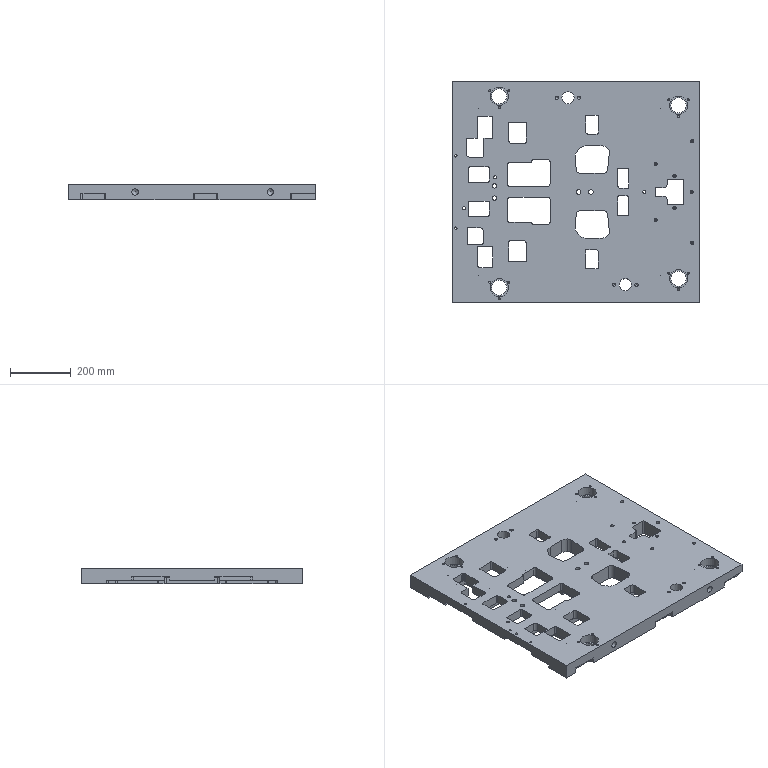Part | STEP file | lll_id14_x_t | 1 solid | 518 faces | box 815 x 730 x 50 mm | volume 21862364 mm3 | cylinder 234 | plane 215 | cone 61 | spline 8 | commonest cylinder face diameters 8 x54 10 x45 8.506 x31 18 x16 6.8 x12 10.5 x7